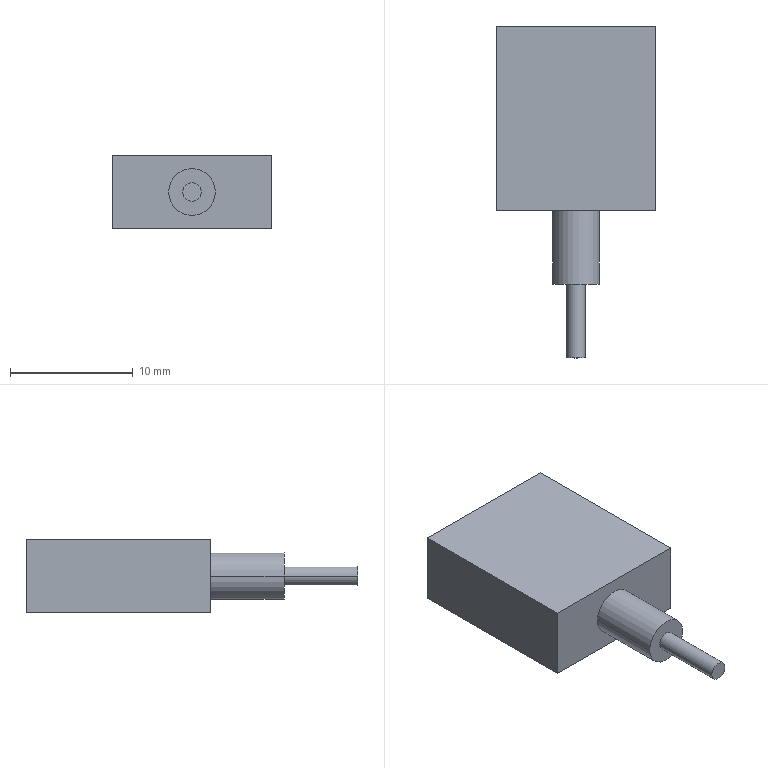Part | STEP file | 0243_015_FPCN14H-1 | 1 solid | 17 faces | box 13 x 27 x 6 mm | volume 1042 mm3 | plane 13 | cylinder 4 | commonest cylinder face diameters 1.5 x2 3.8 x2
STEP:
#1=CARTESIAN_POINT('',(0.,0.,0.));
#2=DIRECTION('',(0.,0.,1.));
#3=DIRECTION('',(1.,0.,0.));
#4=AXIS2_PLACEMENT_3D('',#1,#2,#3);
#5=CARTESIAN_POINT('',(0.75,-27.,3.));
#6=VERTEX_POINT('',#5);
#7=CARTESIAN_POINT('',(-0.75,-27.,3.));
#8=VERTEX_POINT('',#7);
#9=CARTESIAN_POINT('',(0.,-27.,3.));
#10=DIRECTION('',(0.,-1.,0.));
#11=DIRECTION('',(1.,0.,0.));
#12=AXIS2_PLACEMENT_3D('',#9,#10,#11);
#13=CIRCLE('',#12,0.75);
#14=CARTESIAN_POINT('',(0.,-27.,3.));
#15=DIRECTION('',(0.,1.,0.));
#16=DIRECTION('',(-1.,0.,0.));
#17=AXIS2_PLACEMENT_3D('',#14,#15,#16);
#18=CYLINDRICAL_SURFACE('',#17,0.75);
#19=CARTESIAN_POINT('',(3.142,0.));
#20=DIRECTION('',(-1.,0.));
#21=VECTOR('',#20,1.);
#22=LINE('',#19,#21);
#23=(GEOMETRIC_REPRESENTATION_CONTEXT(2)PARAMETRIC_REPRESENTATION_CONTEXT()REPRESENTATION_CONTEXT('',''));
#24=DEFINITIONAL_REPRESENTATION('',(#22),#23);
#25=PCURVE('',#18,#24);
#26=CARTESIAN_POINT('',(0.,-27.,3.));
#27=DIRECTION('',(0.,-1.,0.));
#28=DIRECTION('',(1.,0.,0.));
#29=AXIS2_PLACEMENT_3D('',#26,#27,#28);
#30=PLANE('',#29);
#31=CARTESIAN_POINT('',(0.,0.));
#32=DIRECTION('',(1.,0.));
#33=AXIS2_PLACEMENT_2D('',#31,#32);
#34=CIRCLE('',#33,0.75);
#35=(GEOMETRIC_REPRESENTATION_CONTEXT(2)PARAMETRIC_REPRESENTATION_CONTEXT()REPRESENTATION_CONTEXT('',''));
#36=DEFINITIONAL_REPRESENTATION('',(#34),#35);
#37=PCURVE('',#30,#36);
#38=SURFACE_CURVE('',#13,(#25,#37),.PCURVE_S1.);
#39=EDGE_CURVE('',#6,#8,#38,.T.);
#40=ORIENTED_EDGE('',*,*,#39,.F.);
#41=CARTESIAN_POINT('',(0.75,-21.,3.));
#42=VERTEX_POINT('',#41);
#43=CARTESIAN_POINT('',(0.75,-27.,3.));
#44=DIRECTION('',(0.,1.,0.));
#45=VECTOR('',#44,1.);
#46=LINE('',#43,#45);
#47=CARTESIAN_POINT('',(3.142,0.));
#48=DIRECTION('',(0.,1.));
#49=VECTOR('',#48,1.);
#50=LINE('',#47,#49);
#51=(GEOMETRIC_REPRESENTATION_CONTEXT(2)PARAMETRIC_REPRESENTATION_CONTEXT()REPRESENTATION_CONTEXT('',''));
#52=DEFINITIONAL_REPRESENTATION('',(#50),#51);
#53=PCURVE('',#18,#52);
#54=CARTESIAN_POINT('',(0.,-27.,3.));
#55=DIRECTION('',(0.,1.,0.));
#56=DIRECTION('',(-1.,0.,0.));
#57=AXIS2_PLACEMENT_3D('',#54,#55,#56);
#58=CYLINDRICAL_SURFACE('',#57,0.75);
#59=CARTESIAN_POINT('',(3.142,0.));
#60=DIRECTION('',(0.,1.));
#61=VECTOR('',#60,1.);
#62=LINE('',#59,#61);
#63=(GEOMETRIC_REPRESENTATION_CONTEXT(2)PARAMETRIC_REPRESENTATION_CONTEXT()REPRESENTATION_CONTEXT('',''));
#64=DEFINITIONAL_REPRESENTATION('',(#62),#63);
#65=PCURVE('',#58,#64);
#66=SURFACE_CURVE('',#46,(#53,#65),.PCURVE_S1.);
#67=EDGE_CURVE('',#6,#42,#66,.T.);
#68=ORIENTED_EDGE('',*,*,#67,.T.);
#69=CARTESIAN_POINT('',(-0.75,-21.,3.));
#70=VERTEX_POINT('',#69);
#71=CARTESIAN_POINT('',(0.,-21.,3.));
#72=DIRECTION('',(0.,-1.,0.));
#73=DIRECTION('',(1.,0.,0.));
#74=AXIS2_PLACEMENT_3D('',#71,#72,#73);
#75=CIRCLE('',#74,0.75);
#76=CARTESIAN_POINT('',(3.142,6.));
#77=DIRECTION('',(-1.,0.));
#78=VECTOR('',#77,1.);
#79=LINE('',#76,#78);
#80=(GEOMETRIC_REPRESENTATION_CONTEXT(2)PARAMETRIC_REPRESENTATION_CONTEXT()REPRESENTATION_CONTEXT('',''));
#81=DEFINITIONAL_REPRESENTATION('',(#79),#80);
#82=PCURVE('',#18,#81);
#83=CARTESIAN_POINT('',(0.,-21.,3.));
#84=DIRECTION('',(0.,-1.,0.));
#85=DIRECTION('',(1.,0.,0.));
#86=AXIS2_PLACEMENT_3D('',#83,#84,#85);
#87=PLANE('',#86);
#88=CARTESIAN_POINT('',(0.,0.));
#89=DIRECTION('',(1.,0.));
#90=AXIS2_PLACEMENT_2D('',#88,#89);
#91=CIRCLE('',#90,0.75);
#92=(GEOMETRIC_REPRESENTATION_CONTEXT(2)PARAMETRIC_REPRESENTATION_CONTEXT()REPRESENTATION_CONTEXT('',''));
#93=DEFINITIONAL_REPRESENTATION('',(#91),#92);
#94=PCURVE('',#87,#93);
#95=SURFACE_CURVE('',#75,(#82,#94),.PCURVE_S1.);
#96=EDGE_CURVE('',#42,#70,#95,.T.);
#97=ORIENTED_EDGE('',*,*,#96,.T.);
#98=CARTESIAN_POINT('',(-0.75,-27.,3.));
#99=DIRECTION('',(0.,1.,0.));
#100=VECTOR('',#99,1.);
#101=LINE('',#98,#100);
#102=CARTESIAN_POINT('',(0.,0.));
#103=DIRECTION('',(0.,1.));
#104=VECTOR('',#103,1.);
#105=LINE('',#102,#104);
#106=(GEOMETRIC_REPRESENTATION_CONTEXT(2)PARAMETRIC_REPRESENTATION_CONTEXT()REPRESENTATION_CONTEXT('',''));
#107=DEFINITIONAL_REPRESENTATION('',(#105),#106);
#108=PCURVE('',#18,#107);
#109=CARTESIAN_POINT('',(6.283,0.));
#110=DIRECTION('',(0.,1.));
#111=VECTOR('',#110,1.);
#112=LINE('',#109,#111);
#113=(GEOMETRIC_REPRESENTATION_CONTEXT(2)PARAMETRIC_REPRESENTATION_CONTEXT()REPRESENTATION_CONTEXT('',''));
#114=DEFINITIONAL_REPRESENTATION('',(#112),#113);
#115=PCURVE('',#58,#114);
#116=SURFACE_CURVE('',#101,(#108,#115),.PCURVE_S1.);
#117=EDGE_CURVE('',#8,#70,#116,.T.);
#118=ORIENTED_EDGE('',*,*,#117,.F.);
#119=EDGE_LOOP('',(#40,#68,#97,#118));
#120=FACE_BOUND('',#119,.T.);
#121=ADVANCED_FACE('',(#120),#18,.T.);
#122=CARTESIAN_POINT('',(1.9,-21.,3.));
#123=VERTEX_POINT('',#122);
#124=CARTESIAN_POINT('',(-1.9,-21.,3.));
#125=VERTEX_POINT('',#124);
#126=CARTESIAN_POINT('',(0.,-21.,3.));
#127=DIRECTION('',(0.,-1.,0.));
#128=DIRECTION('',(1.,0.,0.));
#129=AXIS2_PLACEMENT_3D('',#126,#127,#128);
#130=CIRCLE('',#129,1.9);
#131=CARTESIAN_POINT('',(0.,-21.,3.));
#132=DIRECTION('',(0.,1.,0.));
#133=DIRECTION('',(-1.,0.,0.));
#134=AXIS2_PLACEMENT_3D('',#131,#132,#133);
#135=CYLINDRICAL_SURFACE('',#134,1.9);
#136=CARTESIAN_POINT('',(3.142,0.));
#137=DIRECTION('',(-1.,0.));
#138=VECTOR('',#137,1.);
#139=LINE('',#136,#138);
#140=(GEOMETRIC_REPRESENTATION_CONTEXT(2)PARAMETRIC_REPRESENTATION_CONTEXT()REPRESENTATION_CONTEXT('',''));
#141=DEFINITIONAL_REPRESENTATION('',(#139),#140);
#142=PCURVE('',#135,#141);
#143=CARTESIAN_POINT('',(0.,0.));
#144=DIRECTION('',(1.,0.));
#145=AXIS2_PLACEMENT_2D('',#143,#144);
#146=CIRCLE('',#145,1.9);
#147=(GEOMETRIC_REPRESENTATION_CONTEXT(2)PARAMETRIC_REPRESENTATION_CONTEXT()REPRESENTATION_CONTEXT('',''));
#148=DEFINITIONAL_REPRESENTATION('',(#146),#147);
#149=PCURVE('',#87,#148);
#150=SURFACE_CURVE('',#130,(#142,#149),.PCURVE_S1.);
#151=EDGE_CURVE('',#123,#125,#150,.T.);
#152=ORIENTED_EDGE('',*,*,#151,.F.);
#153=CARTESIAN_POINT('',(1.9,-15.,3.));
#154=VERTEX_POINT('',#153);
#155=CARTESIAN_POINT('',(1.9,-21.,3.));
#156=DIRECTION('',(0.,1.,0.));
#157=VECTOR('',#156,1.);
#158=LINE('',#155,#157);
#159=CARTESIAN_POINT('',(3.142,0.));
#160=DIRECTION('',(0.,1.));
#161=VECTOR('',#160,1.);
#162=LINE('',#159,#161);
#163=(GEOMETRIC_REPRESENTATION_CONTEXT(2)PARAMETRIC_REPRESENTATION_CONTEXT()REPRESENTATION_CONTEXT('',''));
#164=DEFINITIONAL_REPRESENTATION('',(#162),#163);
#165=PCURVE('',#135,#164);
#166=CARTESIAN_POINT('',(0.,-21.,3.));
#167=DIRECTION('',(0.,1.,0.));
#168=DIRECTION('',(-1.,0.,0.));
#169=AXIS2_PLACEMENT_3D('',#166,#167,#168);
#170=CYLINDRICAL_SURFACE('',#169,1.9);
#171=CARTESIAN_POINT('',(3.142,0.));
#172=DIRECTION('',(0.,1.));
#173=VECTOR('',#172,1.);
#174=LINE('',#171,#173);
#175=(GEOMETRIC_REPRESENTATION_CONTEXT(2)PARAMETRIC_REPRESENTATION_CONTEXT()REPRESENTATION_CONTEXT('',''));
#176=DEFINITIONAL_REPRESENTATION('',(#174),#175);
#177=PCURVE('',#170,#176);
#178=SURFACE_CURVE('',#158,(#165,#177),.PCURVE_S1.);
#179=EDGE_CURVE('',#123,#154,#178,.T.);
#180=ORIENTED_EDGE('',*,*,#179,.T.);
#181=CARTESIAN_POINT('',(-1.9,-15.,3.));
#182=VERTEX_POINT('',#181);
#183=CARTESIAN_POINT('',(0.,-15.,3.));
#184=DIRECTION('',(0.,-1.,0.));
#185=DIRECTION('',(-1.,0.,0.));
#186=AXIS2_PLACEMENT_3D('',#183,#184,#185);
#187=CIRCLE('',#186,1.9);
#188=CARTESIAN_POINT('',(6.283,6.));
#189=DIRECTION('',(-1.,0.));
#190=VECTOR('',#189,1.);
#191=LINE('',#188,#190);
#192=(GEOMETRIC_REPRESENTATION_CONTEXT(2)PARAMETRIC_REPRESENTATION_CONTEXT()REPRESENTATION_CONTEXT('',''));
#193=DEFINITIONAL_REPRESENTATION('',(#191),#192);
#194=PCURVE('',#135,#193);
#195=CARTESIAN_POINT('',(-6.5,-15.,6.));
#196=DIRECTION('',(0.,1.,0.));
#197=DIRECTION('',(-1.,0.,0.));
#198=AXIS2_PLACEMENT_3D('',#195,#196,#197);
#199=PLANE('',#198);
#200=CARTESIAN_POINT('',(-4.6,-3.));
#201=CARTESIAN_POINT('',(-4.6,-6.291));
#202=CARTESIAN_POINT('',(-7.45,-4.645));
#203=CARTESIAN_POINT('',(-10.3,-3.));
#204=CARTESIAN_POINT('',(-7.45,-1.355));
#205=CARTESIAN_POINT('',(-4.6,0.2909));
#206=CARTESIAN_POINT('',(-4.6,-3.));
#207=(BOUNDED_CURVE()B_SPLINE_CURVE(2,(#200,#201,#202,#203,#204,#205,#206),.UNSPECIFIED.,.T.,.F.)B_SPLINE_CURVE_WITH_KNOTS((1,2,2,2,2,1),(-2.094,0.,2.094,4.189,6.283,8.378),.UNSPECIFIED.)CURVE()GEOMETRIC_REPRESENTATION_ITEM()RATIONAL_B_SPLINE_CURVE((1.,0.5,1.,0.5,1.,0.5,1.))REPRESENTATION_ITEM(''));
#208=(GEOMETRIC_REPRESENTATION_CONTEXT(2)PARAMETRIC_REPRESENTATION_CONTEXT()REPRESENTATION_CONTEXT('',''));
#209=DEFINITIONAL_REPRESENTATION('',(#207),#208);
#210=PCURVE('',#199,#209);
#211=SURFACE_CURVE('',#187,(#194,#210),.PCURVE_S1.);
#212=EDGE_CURVE('',#154,#182,#211,.T.);
#213=ORIENTED_EDGE('',*,*,#212,.T.);
#214=CARTESIAN_POINT('',(-1.9,-21.,3.));
#215=DIRECTION('',(0.,1.,0.));
#216=VECTOR('',#215,1.);
#217=LINE('',#214,#216);
#218=CARTESIAN_POINT('',(0.,0.));
#219=DIRECTION('',(0.,1.));
#220=VECTOR('',#219,1.);
#221=LINE('',#218,#220);
#222=(GEOMETRIC_REPRESENTATION_CONTEXT(2)PARAMETRIC_REPRESENTATION_CONTEXT()REPRESENTATION_CONTEXT('',''));
#223=DEFINITIONAL_REPRESENTATION('',(#221),#222);
#224=PCURVE('',#135,#223);
#225=CARTESIAN_POINT('',(6.283,0.));
#226=DIRECTION('',(0.,1.));
#227=VECTOR('',#226,1.);
#228=LINE('',#225,#227);
#229=(GEOMETRIC_REPRESENTATION_CONTEXT(2)PARAMETRIC_REPRESENTATION_CONTEXT()REPRESENTATION_CONTEXT('',''));
#230=DEFINITIONAL_REPRESENTATION('',(#228),#229);
#231=PCURVE('',#170,#230);
#232=SURFACE_CURVE('',#217,(#224,#231),.PCURVE_S1.);
#233=EDGE_CURVE('',#125,#182,#232,.T.);
#234=ORIENTED_EDGE('',*,*,#233,.F.);
#235=EDGE_LOOP('',(#152,#180,#213,#234));
#236=FACE_BOUND('',#235,.T.);
#237=ADVANCED_FACE('',(#236),#135,.T.);
#238=CARTESIAN_POINT('',(0.,-21.,3.));
#239=DIRECTION('',(0.,-1.,0.));
#240=DIRECTION('',(1.,0.,0.));
#241=AXIS2_PLACEMENT_3D('',#238,#239,#240);
#242=CIRCLE('',#241,1.9);
#243=CARTESIAN_POINT('',(0.,0.));
#244=DIRECTION('',(1.,0.));
#245=AXIS2_PLACEMENT_2D('',#243,#244);
#246=CIRCLE('',#245,1.9);
#247=(GEOMETRIC_REPRESENTATION_CONTEXT(2)PARAMETRIC_REPRESENTATION_CONTEXT()REPRESENTATION_CONTEXT('',''));
#248=DEFINITIONAL_REPRESENTATION('',(#246),#247);
#249=PCURVE('',#87,#248);
#250=CARTESIAN_POINT('',(9.425,0.));
#251=DIRECTION('',(-1.,0.));
#252=VECTOR('',#251,1.);
#253=LINE('',#250,#252);
#254=(GEOMETRIC_REPRESENTATION_CONTEXT(2)PARAMETRIC_REPRESENTATION_CONTEXT()REPRESENTATION_CONTEXT('',''));
#255=DEFINITIONAL_REPRESENTATION('',(#253),#254);
#256=PCURVE('',#170,#255);
#257=SURFACE_CURVE('',#242,(#249,#256),.PCURVE_S1.);
#258=EDGE_CURVE('',#125,#123,#257,.T.);
#259=ORIENTED_EDGE('',*,*,#258,.T.);
#260=ORIENTED_EDGE('',*,*,#151,.T.);
#261=EDGE_LOOP('',(#259,#260));
#262=FACE_BOUND('',#261,.T.);
#263=CARTESIAN_POINT('',(0.,-21.,3.));
#264=DIRECTION('',(0.,-1.,0.));
#265=DIRECTION('',(1.,0.,0.));
#266=AXIS2_PLACEMENT_3D('',#263,#264,#265);
#267=CIRCLE('',#266,0.75);
#268=CARTESIAN_POINT('',(0.,0.));
#269=DIRECTION('',(1.,0.));
#270=AXIS2_PLACEMENT_2D('',#268,#269);
#271=CIRCLE('',#270,0.75);
#272=(GEOMETRIC_REPRESENTATION_CONTEXT(2)PARAMETRIC_REPRESENTATION_CONTEXT()REPRESENTATION_CONTEXT('',''));
#273=DEFINITIONAL_REPRESENTATION('',(#271),#272);
#274=PCURVE('',#87,#273);
#275=CARTESIAN_POINT('',(9.425,6.));
#276=DIRECTION('',(-1.,0.));
#277=VECTOR('',#276,1.);
#278=LINE('',#275,#277);
#279=(GEOMETRIC_REPRESENTATION_CONTEXT(2)PARAMETRIC_REPRESENTATION_CONTEXT()REPRESENTATION_CONTEXT('',''));
#280=DEFINITIONAL_REPRESENTATION('',(#278),#279);
#281=PCURVE('',#58,#280);
#282=SURFACE_CURVE('',#267,(#274,#281),.PCURVE_S1.);
#283=EDGE_CURVE('',#70,#42,#282,.T.);
#284=ORIENTED_EDGE('',*,*,#283,.F.);
#285=ORIENTED_EDGE('',*,*,#96,.F.);
#286=EDGE_LOOP('',(#284,#285));
#287=FACE_BOUND('',#286,.T.);
#288=ADVANCED_FACE('',(#262,#287),#87,.T.);
#289=CARTESIAN_POINT('',(-6.5,-15.,0.));
#290=VERTEX_POINT('',#289);
#291=CARTESIAN_POINT('',(6.5,-15.,0.));
#292=VERTEX_POINT('',#291);
#293=CARTESIAN_POINT('',(-6.5,-15.,0.));
#294=DIRECTION('',(1.,0.,0.));
#295=VECTOR('',#294,1.);
#296=LINE('',#293,#295);
#297=CARTESIAN_POINT('',(0.,-6.));
#298=DIRECTION('',(-1.,0.));
#299=VECTOR('',#298,1.);
#300=LINE('',#297,#299);
#301=(GEOMETRIC_REPRESENTATION_CONTEXT(2)PARAMETRIC_REPRESENTATION_CONTEXT()REPRESENTATION_CONTEXT('',''));
#302=DEFINITIONAL_REPRESENTATION('',(#300),#301);
#303=PCURVE('',#199,#302);
#304=CARTESIAN_POINT('',(-6.5,-15.,0.));
#305=DIRECTION('',(0.,0.,1.));
#306=DIRECTION('',(1.,0.,0.));
#307=AXIS2_PLACEMENT_3D('',#304,#305,#306);
#308=PLANE('',#307);
#309=CARTESIAN_POINT('',(0.,0.));
#310=DIRECTION('',(1.,0.));
#311=VECTOR('',#310,1.);
#312=LINE('',#309,#311);
#313=(GEOMETRIC_REPRESENTATION_CONTEXT(2)PARAMETRIC_REPRESENTATION_CONTEXT()REPRESENTATION_CONTEXT('',''));
#314=DEFINITIONAL_REPRESENTATION('',(#312),#313);
#315=PCURVE('',#308,#314);
#316=SURFACE_CURVE('',#296,(#303,#315),.PCURVE_S1.);
#317=EDGE_CURVE('',#290,#292,#316,.T.);
#318=ORIENTED_EDGE('',*,*,#317,.T.);
#319=CARTESIAN_POINT('',(6.5,-15.,6.));
#320=VERTEX_POINT('',#319);
#321=CARTESIAN_POINT('',(6.5,-15.,6.));
#322=DIRECTION('',(0.,0.,-1.));
#323=VECTOR('',#322,1.);
#324=LINE('',#321,#323);
#325=CARTESIAN_POINT('',(-13.,0.));
#326=DIRECTION('',(0.,-1.));
#327=VECTOR('',#326,1.);
#328=LINE('',#325,#327);
#329=(GEOMETRIC_REPRESENTATION_CONTEXT(2)PARAMETRIC_REPRESENTATION_CONTEXT()REPRESENTATION_CONTEXT('',''));
#330=DEFINITIONAL_REPRESENTATION('',(#328),#329);
#331=PCURVE('',#199,#330);
#332=CARTESIAN_POINT('',(6.5,0.,6.));
#333=DIRECTION('',(-1.,0.,0.));
#334=DIRECTION('',(0.,-1.,0.));
#335=AXIS2_PLACEMENT_3D('',#332,#333,#334);
#336=PLANE('',#335);
#337=CARTESIAN_POINT('',(15.,0.));
#338=DIRECTION('',(0.,-1.));
#339=VECTOR('',#338,1.);
#340=LINE('',#337,#339);
#341=(GEOMETRIC_REPRESENTATION_CONTEXT(2)PARAMETRIC_REPRESENTATION_CONTEXT()REPRESENTATION_CONTEXT('',''));
#342=DEFINITIONAL_REPRESENTATION('',(#340),#341);
#343=PCURVE('',#336,#342);
#344=SURFACE_CURVE('',#324,(#331,#343),.PCURVE_S1.);
#345=EDGE_CURVE('',#320,#292,#344,.T.);
#346=ORIENTED_EDGE('',*,*,#345,.F.);
#347=CARTESIAN_POINT('',(-6.5,-15.,6.));
#348=VERTEX_POINT('',#347);
#349=CARTESIAN_POINT('',(-6.5,-15.,6.));
#350=DIRECTION('',(1.,0.,0.));
#351=VECTOR('',#350,1.);
#352=LINE('',#349,#351);
#353=CARTESIAN_POINT('',(0.,0.));
#354=DIRECTION('',(-1.,0.));
#355=VECTOR('',#354,1.);
#356=LINE('',#353,#355);
#357=(GEOMETRIC_REPRESENTATION_CONTEXT(2)PARAMETRIC_REPRESENTATION_CONTEXT()REPRESENTATION_CONTEXT('',''));
#358=DEFINITIONAL_REPRESENTATION('',(#356),#357);
#359=PCURVE('',#199,#358);
#360=CARTESIAN_POINT('',(-6.5,-15.,6.));
#361=DIRECTION('',(0.,0.,1.));
#362=DIRECTION('',(1.,0.,0.));
#363=AXIS2_PLACEMENT_3D('',#360,#361,#362);
#364=PLANE('',#363);
#365=CARTESIAN_POINT('',(0.,0.));
#366=DIRECTION('',(1.,0.));
#367=VECTOR('',#366,1.);
#368=LINE('',#365,#367);
#369=(GEOMETRIC_REPRESENTATION_CONTEXT(2)PARAMETRIC_REPRESENTATION_CONTEXT()REPRESENTATION_CONTEXT('',''));
#370=DEFINITIONAL_REPRESENTATION('',(#368),#369);
#371=PCURVE('',#364,#370);
#372=SURFACE_CURVE('',#352,(#359,#371),.PCURVE_S1.);
#373=EDGE_CURVE('',#348,#320,#372,.T.);
#374=ORIENTED_EDGE('',*,*,#373,.F.);
#375=CARTESIAN_POINT('',(-6.5,-15.,6.));
#376=DIRECTION('',(0.,0.,-1.));
#377=VECTOR('',#376,1.);
#378=LINE('',#375,#377);
#379=CARTESIAN_POINT('',(0.,0.));
#380=DIRECTION('',(0.,-1.));
#381=VECTOR('',#380,1.);
#382=LINE('',#379,#381);
#383=(GEOMETRIC_REPRESENTATION_CONTEXT(2)PARAMETRIC_REPRESENTATION_CONTEXT()REPRESENTATION_CONTEXT('',''));
#384=DEFINITIONAL_REPRESENTATION('',(#382),#383);
#385=PCURVE('',#199,#384);
#386=CARTESIAN_POINT('',(-6.5,0.,6.));
#387=DIRECTION('',(1.,0.,0.));
#388=DIRECTION('',(0.,1.,0.));
#389=AXIS2_PLACEMENT_3D('',#386,#387,#388);
#390=PLANE('',#389);
#391=CARTESIAN_POINT('',(-15.,0.));
#392=DIRECTION('',(0.,-1.));
#393=VECTOR('',#392,1.);
#394=LINE('',#391,#393);
#395=(GEOMETRIC_REPRESENTATION_CONTEXT(2)PARAMETRIC_REPRESENTATION_CONTEXT()REPRESENTATION_CONTEXT('',''));
#396=DEFINITIONAL_REPRESENTATION('',(#394),#395);
#397=PCURVE('',#390,#396);
#398=SURFACE_CURVE('',#378,(#385,#397),.PCURVE_S1.);
#399=EDGE_CURVE('',#348,#290,#398,.T.);
#400=ORIENTED_EDGE('',*,*,#399,.T.);
#401=EDGE_LOOP('',(#318,#346,#374,#400));
#402=FACE_BOUND('',#401,.T.);
#403=CARTESIAN_POINT('',(0.,-15.,3.));
#404=DIRECTION('',(0.,-1.,0.));
#405=DIRECTION('',(-1.,0.,0.));
#406=AXIS2_PLACEMENT_3D('',#403,#404,#405);
#407=CIRCLE('',#406,1.9);
#408=CARTESIAN_POINT('',(-4.6,-3.));
#409=CARTESIAN_POINT('',(-4.6,-6.291));
#410=CARTESIAN_POINT('',(-7.45,-4.645));
#411=CARTESIAN_POINT('',(-10.3,-3.));
#412=CARTESIAN_POINT('',(-7.45,-1.355));
#413=CARTESIAN_POINT('',(-4.6,0.2909));
#414=CARTESIAN_POINT('',(-4.6,-3.));
#415=(BOUNDED_CURVE()B_SPLINE_CURVE(2,(#408,#409,#410,#411,#412,#413,#414),.UNSPECIFIED.,.T.,.F.)B_SPLINE_CURVE_WITH_KNOTS((1,2,2,2,2,1),(-2.094,0.,2.094,4.189,6.283,8.378),.UNSPECIFIED.)CURVE()GEOMETRIC_REPRESENTATION_ITEM()RATIONAL_B_SPLINE_CURVE((1.,0.5,1.,0.5,1.,0.5,1.))REPRESENTATION_ITEM(''));
#416=(GEOMETRIC_REPRESENTATION_CONTEXT(2)PARAMETRIC_REPRESENTATION_CONTEXT()REPRESENTATION_CONTEXT('',''));
#417=DEFINITIONAL_REPRESENTATION('',(#415),#416);
#418=PCURVE('',#199,#417);
#419=CARTESIAN_POINT('',(6.283,6.));
#420=DIRECTION('',(-1.,0.));
#421=VECTOR('',#420,1.);
#422=LINE('',#419,#421);
#423=(GEOMETRIC_REPRESENTATION_CONTEXT(2)PARAMETRIC_REPRESENTATION_CONTEXT()REPRESENTATION_CONTEXT('',''));
#424=DEFINITIONAL_REPRESENTATION('',(#422),#423);
#425=PCURVE('',#170,#424);
#426=SURFACE_CURVE('',#407,(#418,#425),.PCURVE_S1.);
#427=EDGE_CURVE('',#182,#154,#426,.T.);
#428=ORIENTED_EDGE('',*,*,#427,.F.);
#429=ORIENTED_EDGE('',*,*,#212,.F.);
#430=EDGE_LOOP('',(#428,#429));
#431=FACE_BOUND('',#430,.T.);
#432=ADVANCED_FACE('',(#402,#431),#199,.F.);
#433=CARTESIAN_POINT('',(-6.5,0.,0.));
#434=VERTEX_POINT('',#433);
#435=CARTESIAN_POINT('',(-6.5,0.,0.));
#436=DIRECTION('',(0.,-1.,0.));
#437=VECTOR('',#436,1.);
#438=LINE('',#435,#437);
#439=CARTESIAN_POINT('',(0.,-6.));
#440=DIRECTION('',(-1.,0.));
#441=VECTOR('',#440,1.);
#442=LINE('',#439,#441);
#443=(GEOMETRIC_REPRESENTATION_CONTEXT(2)PARAMETRIC_REPRESENTATION_CONTEXT()REPRESENTATION_CONTEXT('',''));
#444=DEFINITIONAL_REPRESENTATION('',(#442),#443);
#445=PCURVE('',#390,#444);
#446=CARTESIAN_POINT('',(0.,15.));
#447=DIRECTION('',(0.,-1.));
#448=VECTOR('',#447,1.);
#449=LINE('',#446,#448);
#450=(GEOMETRIC_REPRESENTATION_CONTEXT(2)PARAMETRIC_REPRESENTATION_CONTEXT()REPRESENTATION_CONTEXT('',''));
#451=DEFINITIONAL_REPRESENTATION('',(#449),#450);
#452=PCURVE('',#308,#451);
#453=SURFACE_CURVE('',#438,(#445,#452),.PCURVE_S1.);
#454=EDGE_CURVE('',#434,#290,#453,.T.);
#455=ORIENTED_EDGE('',*,*,#454,.T.);
#456=ORIENTED_EDGE('',*,*,#399,.F.);
#457=CARTESIAN_POINT('',(-6.5,0.,6.));
#458=VERTEX_POINT('',#457);
#459=CARTESIAN_POINT('',(-6.5,0.,6.));
#460=DIRECTION('',(0.,-1.,0.));
#461=VECTOR('',#460,1.);
#462=LINE('',#459,#461);
#463=CARTESIAN_POINT('',(0.,0.));
#464=DIRECTION('',(-1.,0.));
#465=VECTOR('',#464,1.);
#466=LINE('',#463,#465);
#467=(GEOMETRIC_REPRESENTATION_CONTEXT(2)PARAMETRIC_REPRESENTATION_CONTEXT()REPRESENTATION_CONTEXT('',''));
#468=DEFINITIONAL_REPRESENTATION('',(#466),#467);
#469=PCURVE('',#390,#468);
#470=CARTESIAN_POINT('',(0.,15.));
#471=DIRECTION('',(0.,-1.));
#472=VECTOR('',#471,1.);
#473=LINE('',#470,#472);
#474=(GEOMETRIC_REPRESENTATION_CONTEXT(2)PARAMETRIC_REPRESENTATION_CONTEXT()REPRESENTATION_CONTEXT('',''));
#475=DEFINITIONAL_REPRESENTATION('',(#473),#474);
#476=PCURVE('',#364,#475);
#477=SURFACE_CURVE('',#462,(#469,#476),.PCURVE_S1.);
#478=EDGE_CURVE('',#458,#348,#477,.T.);
#479=ORIENTED_EDGE('',*,*,#478,.F.);
#480=CARTESIAN_POINT('',(-6.5,0.,6.));
#481=DIRECTION('',(0.,0.,-1.));
#482=VECTOR('',#481,1.);
#483=LINE('',#480,#482);
#484=CARTESIAN_POINT('',(0.,0.));
#485=DIRECTION('',(0.,-1.));
#486=VECTOR('',#485,1.);
#487=LINE('',#484,#486);
#488=(GEOMETRIC_REPRESENTATION_CONTEXT(2)PARAMETRIC_REPRESENTATION_CONTEXT()REPRESENTATION_CONTEXT('',''));
#489=DEFINITIONAL_REPRESENTATION('',(#487),#488);
#490=PCURVE('',#390,#489);
#491=CARTESIAN_POINT('',(-6.5,0.,6.));
#492=DIRECTION('',(0.,-1.,0.));
#493=DIRECTION('',(1.,0.,0.));
#494=AXIS2_PLACEMENT_3D('',#491,#492,#493);
#495=PLANE('',#494);
#496=CARTESIAN_POINT('',(0.,0.));
#497=DIRECTION('',(0.,-1.));
#498=VECTOR('',#497,1.);
#499=LINE('',#496,#498);
#500=(GEOMETRIC_REPRESENTATION_CONTEXT(2)PARAMETRIC_REPRESENTATION_CONTEXT()REPRESENTATION_CONTEXT('',''));
#501=DEFINITIONAL_REPRESENTATION('',(#499),#500);
#502=PCURVE('',#495,#501);
#503=SURFACE_CURVE('',#483,(#490,#502),.PCURVE_S1.);
#504=EDGE_CURVE('',#458,#434,#503,.T.);
#505=ORIENTED_EDGE('',*,*,#504,.T.);
#506=EDGE_LOOP('',(#455,#456,#479,#505));
#507=FACE_BOUND('',#506,.T.);
#508=ADVANCED_FACE('',(#507),#390,.F.);
#509=CARTESIAN_POINT('',(6.5,0.,0.));
#510=VERTEX_POINT('',#509);
#511=CARTESIAN_POINT('',(6.5,0.,0.));
#512=DIRECTION('',(0.,1.,0.));
#513=VECTOR('',#512,1.);
#514=LINE('',#511,#513);
#515=CARTESIAN_POINT('',(0.,-6.));
#516=DIRECTION('',(-1.,0.));
#517=VECTOR('',#516,1.);
#518=LINE('',#515,#517);
#519=(GEOMETRIC_REPRESENTATION_CONTEXT(2)PARAMETRIC_REPRESENTATION_CONTEXT()REPRESENTATION_CONTEXT('',''));
#520=DEFINITIONAL_REPRESENTATION('',(#518),#519);
#521=PCURVE('',#336,#520);
#522=CARTESIAN_POINT('',(13.,15.));
#523=DIRECTION('',(0.,1.));
#524=VECTOR('',#523,1.);
#525=LINE('',#522,#524);
#526=(GEOMETRIC_REPRESENTATION_CONTEXT(2)PARAMETRIC_REPRESENTATION_CONTEXT()REPRESENTATION_CONTEXT('',''));
#527=DEFINITIONAL_REPRESENTATION('',(#525),#526);
#528=PCURVE('',#308,#527);
#529=SURFACE_CURVE('',#514,(#521,#528),.PCURVE_S1.);
#530=EDGE_CURVE('',#292,#510,#529,.T.);
#531=ORIENTED_EDGE('',*,*,#530,.T.);
#532=CARTESIAN_POINT('',(6.5,0.,6.));
#533=VERTEX_POINT('',#532);
#534=CARTESIAN_POINT('',(6.5,0.,6.));
#535=DIRECTION('',(0.,0.,-1.));
#536=VECTOR('',#535,1.);
#537=LINE('',#534,#536);
#538=CARTESIAN_POINT('',(0.,0.));
#539=DIRECTION('',(0.,-1.));
#540=VECTOR('',#539,1.);
#541=LINE('',#538,#540);
#542=(GEOMETRIC_REPRESENTATION_CONTEXT(2)PARAMETRIC_REPRESENTATION_CONTEXT()REPRESENTATION_CONTEXT('',''));
#543=DEFINITIONAL_REPRESENTATION('',(#541),#542);
#544=PCURVE('',#336,#543);
#545=CARTESIAN_POINT('',(13.,0.));
#546=DIRECTION('',(0.,-1.));
#547=VECTOR('',#546,1.);
#548=LINE('',#545,#547);
#549=(GEOMETRIC_REPRESENTATION_CONTEXT(2)PARAMETRIC_REPRESENTATION_CONTEXT()REPRESENTATION_CONTEXT('',''));
#550=DEFINITIONAL_REPRESENTATION('',(#548),#549);
#551=PCURVE('',#495,#550);
#552=SURFACE_CURVE('',#537,(#544,#551),.PCURVE_S1.);
#553=EDGE_CURVE('',#533,#510,#552,.T.);
#554=ORIENTED_EDGE('',*,*,#553,.F.);
#555=CARTESIAN_POINT('',(6.5,0.,6.));
#556=DIRECTION('',(0.,1.,0.));
#557=VECTOR('',#556,1.);
#558=LINE('',#555,#557);
#559=CARTESIAN_POINT('',(0.,0.));
#560=DIRECTION('',(-1.,0.));
#561=VECTOR('',#560,1.);
#562=LINE('',#559,#561);
#563=(GEOMETRIC_REPRESENTATION_CONTEXT(2)PARAMETRIC_REPRESENTATION_CONTEXT()REPRESENTATION_CONTEXT('',''));
#564=DEFINITIONAL_REPRESENTATION('',(#562),#563);
#565=PCURVE('',#336,#564);
#566=CARTESIAN_POINT('',(13.,15.));
#567=DIRECTION('',(0.,1.));
#568=VECTOR('',#567,1.);
#569=LINE('',#566,#568);
#570=(GEOMETRIC_REPRESENTATION_CONTEXT(2)PARAMETRIC_REPRESENTATION_CONTEXT()REPRESENTATION_CONTEXT('',''));
#571=DEFINITIONAL_REPRESENTATION('',(#569),#570);
#572=PCURVE('',#364,#571);
#573=SURFACE_CURVE('',#558,(#565,#572),.PCURVE_S1.);
#574=EDGE_CURVE('',#320,#533,#573,.T.);
#575=ORIENTED_EDGE('',*,*,#574,.F.);
#576=ORIENTED_EDGE('',*,*,#345,.T.);
#577=EDGE_LOOP('',(#531,#554,#575,#576));
#578=FACE_BOUND('',#577,.T.);
#579=ADVANCED_FACE('',(#578),#336,.F.);
#580=CARTESIAN_POINT('',(-6.25,0.,3.4));
#581=VERTEX_POINT('',#580);
#582=CARTESIAN_POINT('',(6.25,0.,3.4));
#583=VERTEX_POINT('',#582);
#584=CARTESIAN_POINT('',(-6.25,0.,3.4));
#585=DIRECTION('',(1.,0.,0.));
#586=VECTOR('',#585,1.);
#587=LINE('',#584,#586);
#588=CARTESIAN_POINT('',(0.25,-2.6));
#589=DIRECTION('',(1.,0.));
#590=VECTOR('',#589,1.);
#591=LINE('',#588,#590);
#592=(GEOMETRIC_REPRESENTATION_CONTEXT(2)PARAMETRIC_REPRESENTATION_CONTEXT()REPRESENTATION_CONTEXT('',''));
#593=DEFINITIONAL_REPRESENTATION('',(#591),#592);
#594=PCURVE('',#495,#593);
#595=CARTESIAN_POINT('',(-6.25,-5.,3.4));
#596=DIRECTION('',(0.,0.,1.));
#597=DIRECTION('',(1.,0.,0.));
#598=AXIS2_PLACEMENT_3D('',#595,#596,#597);
#599=PLANE('',#598);
#600=CARTESIAN_POINT('',(0.,5.));
#601=DIRECTION('',(1.,0.));
#602=VECTOR('',#601,1.);
#603=LINE('',#600,#602);
#604=(GEOMETRIC_REPRESENTATION_CONTEXT(2)PARAMETRIC_REPRESENTATION_CONTEXT()REPRESENTATION_CONTEXT('',''));
#605=DEFINITIONAL_REPRESENTATION('',(#603),#604);
#606=PCURVE('',#599,#605);
#607=SURFACE_CURVE('',#587,(#594,#606),.PCURVE_S1.);
#608=EDGE_CURVE('',#581,#583,#607,.T.);
#609=ORIENTED_EDGE('',*,*,#608,.F.);
#610=CARTESIAN_POINT('',(-6.25,0.,0.1));
#611=VERTEX_POINT('',#610);
#612=CARTESIAN_POINT('',(-6.25,0.,0.1));
#613=DIRECTION('',(0.,0.,1.));
#614=VECTOR('',#613,1.);
#615=LINE('',#612,#614);
#616=CARTESIAN_POINT('',(0.25,-5.9));
#617=DIRECTION('',(0.,1.));
#618=VECTOR('',#617,1.);
#619=LINE('',#616,#618);
#620=(GEOMETRIC_REPRESENTATION_CONTEXT(2)PARAMETRIC_REPRESENTATION_CONTEXT()REPRESENTATION_CONTEXT('',''));
#621=DEFINITIONAL_REPRESENTATION('',(#619),#620);
#622=PCURVE('',#495,#621);
#623=CARTESIAN_POINT('',(-6.25,-5.,0.1));
#624=DIRECTION('',(-1.,0.,0.));
#625=DIRECTION('',(0.,0.,1.));
#626=AXIS2_PLACEMENT_3D('',#623,#624,#625);
#627=PLANE('',#626);
#628=CARTESIAN_POINT('',(0.,5.));
#629=DIRECTION('',(1.,0.));
#630=VECTOR('',#629,1.);
#631=LINE('',#628,#630);
#632=(GEOMETRIC_REPRESENTATION_CONTEXT(2)PARAMETRIC_REPRESENTATION_CONTEXT()REPRESENTATION_CONTEXT('',''));
#633=DEFINITIONAL_REPRESENTATION('',(#631),#632);
#634=PCURVE('',#627,#633);
#635=SURFACE_CURVE('',#615,(#622,#634),.PCURVE_S1.);
#636=EDGE_CURVE('',#611,#581,#635,.T.);
#637=ORIENTED_EDGE('',*,*,#636,.F.);
#638=CARTESIAN_POINT('',(6.25,0.,0.1));
#639=VERTEX_POINT('',#638);
#640=CARTESIAN_POINT('',(-6.25,0.,0.1));
#641=DIRECTION('',(-1.,0.,0.));
#642=VECTOR('',#641,1.);
#643=LINE('',#640,#642);
#644=CARTESIAN_POINT('',(0.25,-5.9));
#645=DIRECTION('',(-1.,0.));
#646=VECTOR('',#645,1.);
#647=LINE('',#644,#646);
#648=(GEOMETRIC_REPRESENTATION_CONTEXT(2)PARAMETRIC_REPRESENTATION_CONTEXT()REPRESENTATION_CONTEXT('',''));
#649=DEFINITIONAL_REPRESENTATION('',(#647),#648);
#650=PCURVE('',#495,#649);
#651=CARTESIAN_POINT('',(-6.25,-5.,0.1));
#652=DIRECTION('',(0.,0.,-1.));
#653=DIRECTION('',(-1.,0.,0.));
#654=AXIS2_PLACEMENT_3D('',#651,#652,#653);
#655=PLANE('',#654);
#656=CARTESIAN_POINT('',(0.,5.));
#657=DIRECTION('',(1.,0.));
#658=VECTOR('',#657,1.);
#659=LINE('',#656,#658);
#660=(GEOMETRIC_REPRESENTATION_CONTEXT(2)PARAMETRIC_REPRESENTATION_CONTEXT()REPRESENTATION_CONTEXT('',''));
#661=DEFINITIONAL_REPRESENTATION('',(#659),#660);
#662=PCURVE('',#655,#661);
#663=SURFACE_CURVE('',#643,(#650,#662),.PCURVE_S1.);
#664=EDGE_CURVE('',#639,#611,#663,.T.);
#665=ORIENTED_EDGE('',*,*,#664,.F.);
#666=CARTESIAN_POINT('',(6.25,0.,0.1));
#667=DIRECTION('',(0.,0.,-1.));
#668=VECTOR('',#667,1.);
#669=LINE('',#666,#668);
#670=CARTESIAN_POINT('',(12.75,-5.9));
#671=DIRECTION('',(0.,-1.));
#672=VECTOR('',#671,1.);
#673=LINE('',#670,#672);
#674=(GEOMETRIC_REPRESENTATION_CONTEXT(2)PARAMETRIC_REPRESENTATION_CONTEXT()REPRESENTATION_CONTEXT('',''));
#675=DEFINITIONAL_REPRESENTATION('',(#673),#674);
#676=PCURVE('',#495,#675);
#677=CARTESIAN_POINT('',(6.25,-5.,0.1));
#678=DIRECTION('',(1.,0.,0.));
#679=DIRECTION('',(0.,1.,0.));
#680=AXIS2_PLACEMENT_3D('',#677,#678,#679);
#681=PLANE('',#680);
#682=CARTESIAN_POINT('',(5.,0.));
#683=DIRECTION('',(0.,-1.));
#684=VECTOR('',#683,1.);
#685=LINE('',#682,#684);
#686=(GEOMETRIC_REPRESENTATION_CONTEXT(2)PARAMETRIC_REPRESENTATION_CONTEXT()REPRESENTATION_CONTEXT('',''));
#687=DEFINITIONAL_REPRESENTATION('',(#685),#686);
#688=PCURVE('',#681,#687);
#689=SURFACE_CURVE('',#669,(#676,#688),.PCURVE_S1.);
#690=EDGE_CURVE('',#583,#639,#689,.T.);
#691=ORIENTED_EDGE('',*,*,#690,.F.);
#692=EDGE_LOOP('',(#609,#637,#665,#691));
#693=FACE_BOUND('',#692,.T.);
#694=CARTESIAN_POINT('',(-6.5,0.,0.));
#695=DIRECTION('',(-1.,0.,0.));
#696=VECTOR('',#695,1.);
#697=LINE('',#694,#696);
#698=CARTESIAN_POINT('',(0.,-6.));
#699=DIRECTION('',(-1.,0.));
#700=VECTOR('',#699,1.);
#701=LINE('',#698,#700);
#702=(GEOMETRIC_REPRESENTATION_CONTEXT(2)PARAMETRIC_REPRESENTATION_CONTEXT()REPRESENTATION_CONTEXT('',''));
#703=DEFINITIONAL_REPRESENTATION('',(#701),#702);
#704=PCURVE('',#495,#703);
#705=CARTESIAN_POINT('',(0.,15.));
#706=DIRECTION('',(-1.,0.));
#707=VECTOR('',#706,1.);
#708=LINE('',#705,#707);
#709=(GEOMETRIC_REPRESENTATION_CONTEXT(2)PARAMETRIC_REPRESENTATION_CONTEXT()REPRESENTATION_CONTEXT('',''));
#710=DEFINITIONAL_REPRESENTATION('',(#708),#709);
#711=PCURVE('',#308,#710);
#712=SURFACE_CURVE('',#697,(#704,#711),.PCURVE_S1.);
#713=EDGE_CURVE('',#510,#434,#712,.T.);
#714=ORIENTED_EDGE('',*,*,#713,.T.);
#715=ORIENTED_EDGE('',*,*,#504,.F.);
#716=CARTESIAN_POINT('',(-6.5,0.,6.));
#717=DIRECTION('',(-1.,0.,0.));
#718=VECTOR('',#717,1.);
#719=LINE('',#716,#718);
#720=CARTESIAN_POINT('',(0.,0.));
#721=DIRECTION('',(-1.,0.));
#722=VECTOR('',#721,1.);
#723=LINE('',#720,#722);
#724=(GEOMETRIC_REPRESENTATION_CONTEXT(2)PARAMETRIC_REPRESENTATION_CONTEXT()REPRESENTATION_CONTEXT('',''));
#725=DEFINITIONAL_REPRESENTATION('',(#723),#724);
#726=PCURVE('',#495,#725);
#727=CARTESIAN_POINT('',(0.,15.));
#728=DIRECTION('',(-1.,0.));
#729=VECTOR('',#728,1.);
#730=LINE('',#727,#729);
#731=(GEOMETRIC_REPRESENTATION_CONTEXT(2)PARAMETRIC_REPRESENTATION_CONTEXT()REPRESENTATION_CONTEXT('',''));
#732=DEFINITIONAL_REPRESENTATION('',(#730),#731);
#733=PCURVE('',#364,#732);
#734=SURFACE_CURVE('',#719,(#726,#733),.PCURVE_S1.);
#735=EDGE_CURVE('',#533,#458,#734,.T.);
#736=ORIENTED_EDGE('',*,*,#735,.F.);
#737=ORIENTED_EDGE('',*,*,#553,.T.);
#738=EDGE_LOOP('',(#714,#715,#736,#737));
#739=FACE_BOUND('',#738,.T.);
#740=ADVANCED_FACE('',(#693,#739),#495,.F.);
#741=ORIENTED_EDGE('',*,*,#478,.T.);
#742=ORIENTED_EDGE('',*,*,#373,.T.);
#743=ORIENTED_EDGE('',*,*,#574,.T.);
#744=ORIENTED_EDGE('',*,*,#735,.T.);
#745=EDGE_LOOP('',(#741,#742,#743,#744));
#746=FACE_BOUND('',#745,.T.);
#747=ADVANCED_FACE('',(#746),#364,.T.);
#748=ORIENTED_EDGE('',*,*,#454,.F.);
#749=ORIENTED_EDGE('',*,*,#713,.F.);
#750=ORIENTED_EDGE('',*,*,#530,.F.);
#751=ORIENTED_EDGE('',*,*,#317,.F.);
#752=EDGE_LOOP('',(#748,#749,#750,#751));
#753=FACE_BOUND('',#752,.T.);
#754=ADVANCED_FACE('',(#753),#308,.F.);
#755=ORIENTED_EDGE('',*,*,#179,.F.);
#756=ORIENTED_EDGE('',*,*,#258,.F.);
#757=ORIENTED_EDGE('',*,*,#233,.T.);
#758=ORIENTED_EDGE('',*,*,#427,.T.);
#759=EDGE_LOOP('',(#755,#756,#757,#758));
#760=FACE_BOUND('',#759,.T.);
#761=ADVANCED_FACE('',(#760),#170,.T.);
#762=ORIENTED_EDGE('',*,*,#67,.F.);
#763=CARTESIAN_POINT('',(0.,-27.,3.));
#764=DIRECTION('',(0.,-1.,0.));
#765=DIRECTION('',(1.,0.,0.));
#766=AXIS2_PLACEMENT_3D('',#763,#764,#765);
#767=CIRCLE('',#766,0.75);
#768=CARTESIAN_POINT('',(9.425,0.));
#769=DIRECTION('',(-1.,0.));
#770=VECTOR('',#769,1.);
#771=LINE('',#768,#770);
#772=(GEOMETRIC_REPRESENTATION_CONTEXT(2)PARAMETRIC_REPRESENTATION_CONTEXT()REPRESENTATION_CONTEXT('',''));
#773=DEFINITIONAL_REPRESENTATION('',(#771),#772);
#774=PCURVE('',#58,#773);
#775=CARTESIAN_POINT('',(0.,0.));
#776=DIRECTION('',(1.,0.));
#777=AXIS2_PLACEMENT_2D('',#775,#776);
#778=CIRCLE('',#777,0.75);
#779=(GEOMETRIC_REPRESENTATION_CONTEXT(2)PARAMETRIC_REPRESENTATION_CONTEXT()REPRESENTATION_CONTEXT('',''));
#780=DEFINITIONAL_REPRESENTATION('',(#778),#779);
#781=PCURVE('',#30,#780);
#782=SURFACE_CURVE('',#767,(#774,#781),.PCURVE_S1.);
#783=EDGE_CURVE('',#8,#6,#782,.T.);
#784=ORIENTED_EDGE('',*,*,#783,.F.);
#785=ORIENTED_EDGE('',*,*,#117,.T.);
#786=ORIENTED_EDGE('',*,*,#283,.T.);
#787=EDGE_LOOP('',(#762,#784,#785,#786));
#788=FACE_BOUND('',#787,.T.);
#789=ADVANCED_FACE('',(#788),#58,.T.);
#790=ORIENTED_EDGE('',*,*,#783,.T.);
#791=ORIENTED_EDGE('',*,*,#39,.T.);
#792=EDGE_LOOP('',(#790,#791));
#793=FACE_BOUND('',#792,.T.);
#794=ADVANCED_FACE('',(#793),#30,.T.);
#795=ORIENTED_EDGE('',*,*,#636,.T.);
#796=CARTESIAN_POINT('',(-6.25,-5.,3.4));
#797=VERTEX_POINT('',#796);
#798=CARTESIAN_POINT('',(-6.25,-5.,3.4));
#799=DIRECTION('',(0.,1.,0.));
#800=VECTOR('',#799,1.);
#801=LINE('',#798,#800);
#802=CARTESIAN_POINT('',(3.3,0.));
#803=DIRECTION('',(0.,1.));
#804=VECTOR('',#803,1.);
#805=LINE('',#802,#804);
#806=(GEOMETRIC_REPRESENTATION_CONTEXT(2)PARAMETRIC_REPRESENTATION_CONTEXT()REPRESENTATION_CONTEXT('',''));
#807=DEFINITIONAL_REPRESENTATION('',(#805),#806);
#808=PCURVE('',#627,#807);
#809=CARTESIAN_POINT('',(0.,0.));
#810=DIRECTION('',(0.,1.));
#811=VECTOR('',#810,1.);
#812=LINE('',#809,#811);
#813=(GEOMETRIC_REPRESENTATION_CONTEXT(2)PARAMETRIC_REPRESENTATION_CONTEXT()REPRESENTATION_CONTEXT('',''));
#814=DEFINITIONAL_REPRESENTATION('',(#812),#813);
#815=PCURVE('',#599,#814);
#816=SURFACE_CURVE('',#801,(#808,#815),.PCURVE_S1.);
#817=EDGE_CURVE('',#797,#581,#816,.T.);
#818=ORIENTED_EDGE('',*,*,#817,.F.);
#819=CARTESIAN_POINT('',(-6.25,-5.,0.1));
#820=VERTEX_POINT('',#819);
#821=CARTESIAN_POINT('',(-6.25,-5.,0.1));
#822=DIRECTION('',(0.,0.,1.));
#823=VECTOR('',#822,1.);
#824=LINE('',#821,#823);
#825=CARTESIAN_POINT('',(0.,0.));
#826=DIRECTION('',(1.,0.));
#827=VECTOR('',#826,1.);
#828=LINE('',#825,#827);
#829=(GEOMETRIC_REPRESENTATION_CONTEXT(2)PARAMETRIC_REPRESENTATION_CONTEXT()REPRESENTATION_CONTEXT('',''));
#830=DEFINITIONAL_REPRESENTATION('',(#828),#829);
#831=PCURVE('',#627,#830);
#832=CARTESIAN_POINT('',(-6.25,-5.,3.4));
#833=DIRECTION('',(0.,1.,0.));
#834=DIRECTION('',(-1.,0.,0.));
#835=AXIS2_PLACEMENT_3D('',#832,#833,#834);
#836=PLANE('',#835);
#837=CARTESIAN_POINT('',(0.,-3.3));
#838=DIRECTION('',(0.,1.));
#839=VECTOR('',#838,1.);
#840=LINE('',#837,#839);
#841=(GEOMETRIC_REPRESENTATION_CONTEXT(2)PARAMETRIC_REPRESENTATION_CONTEXT()REPRESENTATION_CONTEXT('',''));
#842=DEFINITIONAL_REPRESENTATION('',(#840),#841);
#843=PCURVE('',#836,#842);
#844=SURFACE_CURVE('',#824,(#831,#843),.PCURVE_S1.);
#845=EDGE_CURVE('',#820,#797,#844,.T.);
#846=ORIENTED_EDGE('',*,*,#845,.F.);
#847=CARTESIAN_POINT('',(-6.25,-5.,0.1));
#848=DIRECTION('',(0.,1.,0.));
#849=VECTOR('',#848,1.);
#850=LINE('',#847,#849);
#851=CARTESIAN_POINT('',(0.,0.));
#852=DIRECTION('',(0.,1.));
#853=VECTOR('',#852,1.);
#854=LINE('',#851,#853);
#855=(GEOMETRIC_REPRESENTATION_CONTEXT(2)PARAMETRIC_REPRESENTATION_CONTEXT()REPRESENTATION_CONTEXT('',''));
#856=DEFINITIONAL_REPRESENTATION('',(#854),#855);
#857=PCURVE('',#627,#856);
#858=CARTESIAN_POINT('',(0.,0.));
#859=DIRECTION('',(0.,1.));
#860=VECTOR('',#859,1.);
#861=LINE('',#858,#860);
#862=(GEOMETRIC_REPRESENTATION_CONTEXT(2)PARAMETRIC_REPRESENTATION_CONTEXT()REPRESENTATION_CONTEXT('',''));
#863=DEFINITIONAL_REPRESENTATION('',(#861),#862);
#864=PCURVE('',#655,#863);
#865=SURFACE_CURVE('',#850,(#857,#864),.PCURVE_S1.);
#866=EDGE_CURVE('',#820,#611,#865,.T.);
#867=ORIENTED_EDGE('',*,*,#866,.T.);
#868=EDGE_LOOP('',(#795,#818,#846,#867));
#869=FACE_BOUND('',#868,.T.);
#870=ADVANCED_FACE('',(#869),#627,.F.);
#871=ORIENTED_EDGE('',*,*,#664,.T.);
#872=ORIENTED_EDGE('',*,*,#866,.F.);
#873=CARTESIAN_POINT('',(6.25,-5.,0.1));
#874=VERTEX_POINT('',#873);
#875=CARTESIAN_POINT('',(-6.25,-5.,0.1));
#876=DIRECTION('',(-1.,0.,0.));
#877=VECTOR('',#876,1.);
#878=LINE('',#875,#877);
#879=CARTESIAN_POINT('',(0.,0.));
#880=DIRECTION('',(1.,0.));
#881=VECTOR('',#880,1.);
#882=LINE('',#879,#881);
#883=(GEOMETRIC_REPRESENTATION_CONTEXT(2)PARAMETRIC_REPRESENTATION_CONTEXT()REPRESENTATION_CONTEXT('',''));
#884=DEFINITIONAL_REPRESENTATION('',(#882),#883);
#885=PCURVE('',#655,#884);
#886=CARTESIAN_POINT('',(0.,-3.3));
#887=DIRECTION('',(1.,0.));
#888=VECTOR('',#887,1.);
#889=LINE('',#886,#888);
#890=(GEOMETRIC_REPRESENTATION_CONTEXT(2)PARAMETRIC_REPRESENTATION_CONTEXT()REPRESENTATION_CONTEXT('',''));
#891=DEFINITIONAL_REPRESENTATION('',(#889),#890);
#892=PCURVE('',#836,#891);
#893=SURFACE_CURVE('',#878,(#885,#892),.PCURVE_S1.);
#894=EDGE_CURVE('',#874,#820,#893,.T.);
#895=ORIENTED_EDGE('',*,*,#894,.F.);
#896=CARTESIAN_POINT('',(6.25,-5.,0.1));
#897=DIRECTION('',(0.,1.,0.));
#898=VECTOR('',#897,1.);
#899=LINE('',#896,#898);
#900=CARTESIAN_POINT('',(-12.5,0.));
#901=DIRECTION('',(0.,1.));
#902=VECTOR('',#901,1.);
#903=LINE('',#900,#902);
#904=(GEOMETRIC_REPRESENTATION_CONTEXT(2)PARAMETRIC_REPRESENTATION_CONTEXT()REPRESENTATION_CONTEXT('',''));
#905=DEFINITIONAL_REPRESENTATION('',(#903),#904);
#906=PCURVE('',#655,#905);
#907=CARTESIAN_POINT('',(0.,0.));
#908=DIRECTION('',(1.,0.));
#909=VECTOR('',#908,1.);
#910=LINE('',#907,#909);
#911=(GEOMETRIC_REPRESENTATION_CONTEXT(2)PARAMETRIC_REPRESENTATION_CONTEXT()REPRESENTATION_CONTEXT('',''));
#912=DEFINITIONAL_REPRESENTATION('',(#910),#911);
#913=PCURVE('',#681,#912);
#914=SURFACE_CURVE('',#899,(#906,#913),.PCURVE_S1.);
#915=EDGE_CURVE('',#874,#639,#914,.T.);
#916=ORIENTED_EDGE('',*,*,#915,.T.);
#917=EDGE_LOOP('',(#871,#872,#895,#916));
#918=FACE_BOUND('',#917,.T.);
#919=ADVANCED_FACE('',(#918),#655,.F.);
#920=ORIENTED_EDGE('',*,*,#690,.T.);
#921=ORIENTED_EDGE('',*,*,#915,.F.);
#922=CARTESIAN_POINT('',(6.25,-5.,3.4));
#923=VERTEX_POINT('',#922);
#924=CARTESIAN_POINT('',(6.25,-5.,0.1));
#925=DIRECTION('',(0.,0.,-1.));
#926=VECTOR('',#925,1.);
#927=LINE('',#924,#926);
#928=CARTESIAN_POINT('',(0.,0.));
#929=DIRECTION('',(0.,-1.));
#930=VECTOR('',#929,1.);
#931=LINE('',#928,#930);
#932=(GEOMETRIC_REPRESENTATION_CONTEXT(2)PARAMETRIC_REPRESENTATION_CONTEXT()REPRESENTATION_CONTEXT('',''));
#933=DEFINITIONAL_REPRESENTATION('',(#931),#932);
#934=PCURVE('',#681,#933);
#935=CARTESIAN_POINT('',(-12.5,-3.3));
#936=DIRECTION('',(0.,-1.));
#937=VECTOR('',#936,1.);
#938=LINE('',#935,#937);
#939=(GEOMETRIC_REPRESENTATION_CONTEXT(2)PARAMETRIC_REPRESENTATION_CONTEXT()REPRESENTATION_CONTEXT('',''));
#940=DEFINITIONAL_REPRESENTATION('',(#938),#939);
#941=PCURVE('',#836,#940);
#942=SURFACE_CURVE('',#927,(#934,#941),.PCURVE_S1.);
#943=EDGE_CURVE('',#923,#874,#942,.T.);
#944=ORIENTED_EDGE('',*,*,#943,.F.);
#945=CARTESIAN_POINT('',(6.25,-5.,3.4));
#946=DIRECTION('',(0.,1.,0.));
#947=VECTOR('',#946,1.);
#948=LINE('',#945,#947);
#949=CARTESIAN_POINT('',(0.,3.3));
#950=DIRECTION('',(1.,0.));
#951=VECTOR('',#950,1.);
#952=LINE('',#949,#951);
#953=(GEOMETRIC_REPRESENTATION_CONTEXT(2)PARAMETRIC_REPRESENTATION_CONTEXT()REPRESENTATION_CONTEXT('',''));
#954=DEFINITIONAL_REPRESENTATION('',(#952),#953);
#955=PCURVE('',#681,#954);
#956=CARTESIAN_POINT('',(12.5,0.));
#957=DIRECTION('',(0.,1.));
#958=VECTOR('',#957,1.);
#959=LINE('',#956,#958);
#960=(GEOMETRIC_REPRESENTATION_CONTEXT(2)PARAMETRIC_REPRESENTATION_CONTEXT()REPRESENTATION_CONTEXT('',''));
#961=DEFINITIONAL_REPRESENTATION('',(#959),#960);
#962=PCURVE('',#599,#961);
#963=SURFACE_CURVE('',#948,(#955,#962),.PCURVE_S1.);
#964=EDGE_CURVE('',#923,#583,#963,.T.);
#965=ORIENTED_EDGE('',*,*,#964,.T.);
#966=EDGE_LOOP('',(#920,#921,#944,#965));
#967=FACE_BOUND('',#966,.T.);
#968=ADVANCED_FACE('',(#967),#681,.F.);
#969=ORIENTED_EDGE('',*,*,#608,.T.);
#970=ORIENTED_EDGE('',*,*,#964,.F.);
#971=CARTESIAN_POINT('',(-6.25,-5.,3.4));
#972=DIRECTION('',(1.,0.,0.));
#973=VECTOR('',#972,1.);
#974=LINE('',#971,#973);
#975=CARTESIAN_POINT('',(0.,0.));
#976=DIRECTION('',(1.,0.));
#977=VECTOR('',#976,1.);
#978=LINE('',#975,#977);
#979=(GEOMETRIC_REPRESENTATION_CONTEXT(2)PARAMETRIC_REPRESENTATION_CONTEXT()REPRESENTATION_CONTEXT('',''));
#980=DEFINITIONAL_REPRESENTATION('',(#978),#979);
#981=PCURVE('',#599,#980);
#982=CARTESIAN_POINT('',(0.,0.));
#983=DIRECTION('',(-1.,0.));
#984=VECTOR('',#983,1.);
#985=LINE('',#982,#984);
#986=(GEOMETRIC_REPRESENTATION_CONTEXT(2)PARAMETRIC_REPRESENTATION_CONTEXT()REPRESENTATION_CONTEXT('',''));
#987=DEFINITIONAL_REPRESENTATION('',(#985),#986);
#988=PCURVE('',#836,#987);
#989=SURFACE_CURVE('',#974,(#981,#988),.PCURVE_S1.);
#990=EDGE_CURVE('',#797,#923,#989,.T.);
#991=ORIENTED_EDGE('',*,*,#990,.F.);
#992=ORIENTED_EDGE('',*,*,#817,.T.);
#993=EDGE_LOOP('',(#969,#970,#991,#992));
#994=FACE_BOUND('',#993,.T.);
#995=ADVANCED_FACE('',(#994),#599,.F.);
#996=ORIENTED_EDGE('',*,*,#845,.T.);
#997=ORIENTED_EDGE('',*,*,#990,.T.);
#998=ORIENTED_EDGE('',*,*,#943,.T.);
#999=ORIENTED_EDGE('',*,*,#894,.T.);
#1000=EDGE_LOOP('',(#996,#997,#998,#999));
#1001=FACE_BOUND('',#1000,.T.);
#1002=ADVANCED_FACE('',(#1001),#836,.T.);
#1003=CLOSED_SHELL('',(#121,#237,#288,#432,#508,#579,#740,#747,#754,#761,#789,#794,#870,#919,#968,#995,#1002));
#1004=MANIFOLD_SOLID_BREP('',#1003);
#1005=(LENGTH_UNIT()NAMED_UNIT(*)SI_UNIT(.MILLI.,.METRE.));
#1006=UNCERTAINTY_MEASURE_WITH_UNIT(LENGTH_MEASURE(0.0000001),#1005,'','');
#1007=(NAMED_UNIT(*)PLANE_ANGLE_UNIT()SI_UNIT($,.RADIAN.));
#1008=(NAMED_UNIT(*)SI_UNIT($,.STERADIAN.)SOLID_ANGLE_UNIT());
#1009=(GEOMETRIC_REPRESENTATION_CONTEXT(3)GLOBAL_UNCERTAINTY_ASSIGNED_CONTEXT((#1006))GLOBAL_UNIT_ASSIGNED_CONTEXT((#1005,#1007,#1008))REPRESENTATION_CONTEXT('',''));
#1010=ADVANCED_BREP_SHAPE_REPRESENTATION('',(#4,#1004),#1009);